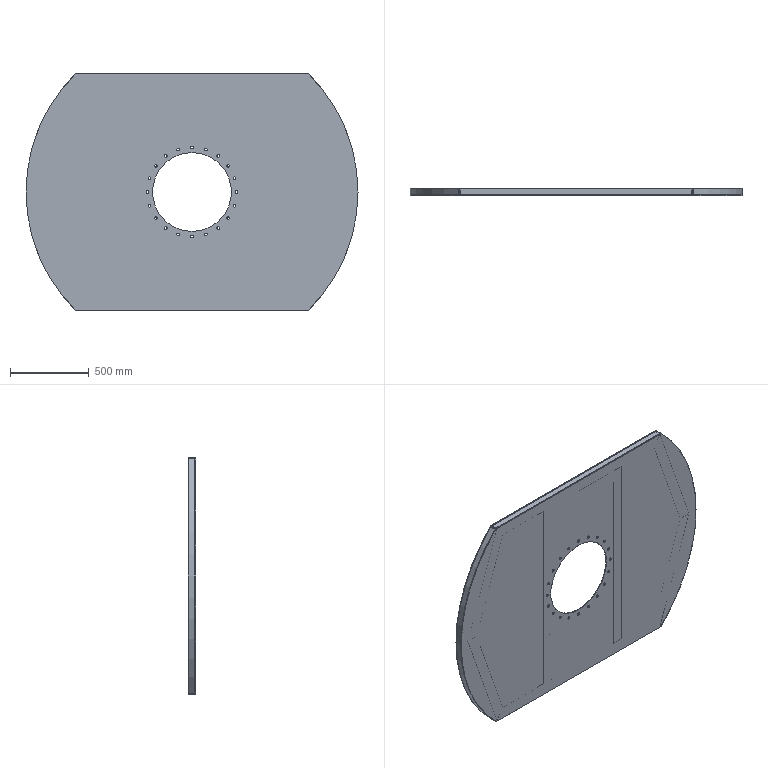Part | STEP file | 7-Roller base_default<machined> | 14 solids | 334 faces | box 2105 x 48 x 1497 mm | volume 25567908 mm3 | cylinder 198 | plane 120 | cone 16 | commonest cylinder face diameters 2 x40 6 x40 17 x40 6.8 x36 5 x32 2105 x6